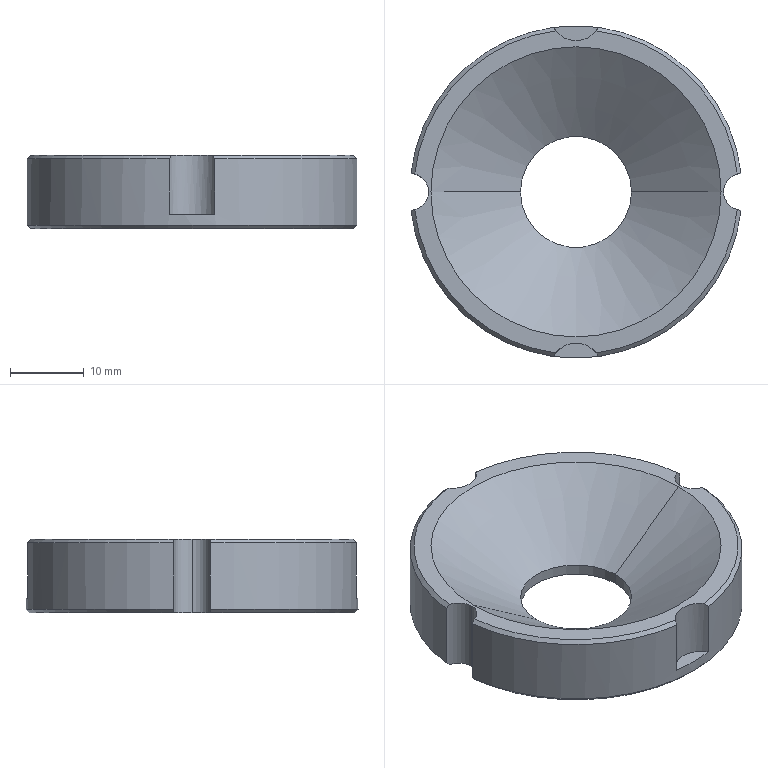Part | STEP file | 10000020561swp000-1 | 1 solid | 21 faces | box 44.722 x 45 x 10 mm | volume 10014 mm3 | cylinder 9 | cone 8 | plane 4 | commonest cylinder face diameters 5 x3 7 x2 15.05 x2 45 x2
STEP:
#1=CARTESIAN_POINT('',(7.525,0.,1.5));
#2=VERTEX_POINT('',#1);
#3=CARTESIAN_POINT('',(-7.525,0.,1.5));
#4=VERTEX_POINT('',#3);
#5=CARTESIAN_POINT('',(0.,0.,1.5));
#6=DIRECTION('',(0.,0.,-1.));
#7=DIRECTION('',(-1.,0.,0.));
#8=AXIS2_PLACEMENT_3D('',#5,#6,#7);
#9=CIRCLE('',#8,7.525);
#10=EDGE_CURVE('',#2,#4,#9,.T.);
#11=ORIENTED_EDGE('',*,*,#10,.T.);
#12=CARTESIAN_POINT('',(-19.664,0.,10.));
#13=VERTEX_POINT('',#12);
#14=CARTESIAN_POINT('',(-7.525,0.,1.5));
#15=DIRECTION('',(-0.8192,0.,0.5736));
#16=VECTOR('',#15,1000.);
#17=LINE('',#14,#16);
#18=EDGE_CURVE('',#4,#13,#17,.T.);
#19=ORIENTED_EDGE('',*,*,#18,.T.);
#20=CARTESIAN_POINT('',(19.664,0.,10.));
#21=VERTEX_POINT('',#20);
#22=CARTESIAN_POINT('',(0.,0.,10.));
#23=DIRECTION('',(0.,0.,-1.));
#24=DIRECTION('',(-1.,0.,0.));
#25=AXIS2_PLACEMENT_3D('',#22,#23,#24);
#26=CIRCLE('',#25,19.664);
#27=EDGE_CURVE('',#21,#13,#26,.T.);
#28=ORIENTED_EDGE('',*,*,#27,.F.);
#29=CARTESIAN_POINT('',(7.525,0.,1.5));
#30=DIRECTION('',(0.8192,0.,0.5736));
#31=VECTOR('',#30,1000.);
#32=LINE('',#29,#31);
#33=EDGE_CURVE('',#2,#21,#32,.T.);
#34=ORIENTED_EDGE('',*,*,#33,.F.);
#35=EDGE_LOOP('',(#11,#19,#28,#34));
#36=FACE_OUTER_BOUND('',#35,.T.);
#37=CARTESIAN_POINT('',(0.,0.,1.5));
#38=DIRECTION('',(0.,0.,1.));
#39=DIRECTION('',(1.,0.,0.));
#40=AXIS2_PLACEMENT_3D('',#37,#38,#39);
#41=CONICAL_SURFACE('',#40,7.525,0.9599);
#42=ADVANCED_FACE('',(#36),#41,.F.);
#43=CARTESIAN_POINT('',(-20.,0.,0.));
#44=VERTEX_POINT('',#43);
#45=CARTESIAN_POINT('',(-21.867,2.418,0.));
#46=VERTEX_POINT('',#45);
#47=CARTESIAN_POINT('',(-22.5,0.,0.));
#48=DIRECTION('',(0.,0.,1.));
#49=DIRECTION('',(1.,0.,0.));
#50=AXIS2_PLACEMENT_3D('',#47,#48,#49);
#51=CIRCLE('',#50,2.5);
#52=EDGE_CURVE('',#44,#46,#51,.T.);
#53=ORIENTED_EDGE('',*,*,#52,.F.);
#54=CARTESIAN_POINT('',(-20.,0.,10.));
#55=VERTEX_POINT('',#54);
#56=CARTESIAN_POINT('',(-20.,0.,0.));
#57=DIRECTION('',(0.,0.,1.));
#58=VECTOR('',#57,1000.);
#59=LINE('',#56,#58);
#60=EDGE_CURVE('',#44,#55,#59,.T.);
#61=ORIENTED_EDGE('',*,*,#60,.T.);
#62=CARTESIAN_POINT('',(-21.867,2.418,10.));
#63=VERTEX_POINT('',#62);
#64=CARTESIAN_POINT('',(-22.5,0.,10.));
#65=DIRECTION('',(0.,0.,1.));
#66=DIRECTION('',(1.,0.,0.));
#67=AXIS2_PLACEMENT_3D('',#64,#65,#66);
#68=CIRCLE('',#67,2.5);
#69=EDGE_CURVE('',#55,#63,#68,.T.);
#70=ORIENTED_EDGE('',*,*,#69,.T.);
#71=CARTESIAN_POINT('',(-22.361,2.496,9.5));
#72=VERTEX_POINT('',#71);
#73=CARTESIAN_POINT('',(-21.867,2.418,10.));
#74=CARTESIAN_POINT('',(-22.029,2.461,9.834));
#75=CARTESIAN_POINT('',(-22.194,2.487,9.667));
#76=CARTESIAN_POINT('',(-22.361,2.496,9.5));
#77=B_SPLINE_CURVE_WITH_KNOTS('',3,(#73,#74,#75,#76),.UNSPECIFIED.,.F.,.F.,(4,4),(0.,0.0007075),.UNSPECIFIED.);
#78=EDGE_CURVE('',#63,#72,#77,.T.);
#79=ORIENTED_EDGE('',*,*,#78,.T.);
#80=CARTESIAN_POINT('',(-22.361,2.496,0.5));
#81=VERTEX_POINT('',#80);
#82=CARTESIAN_POINT('',(-22.361,2.496,5.));
#83=DIRECTION('',(0.,0.,1.));
#84=VECTOR('',#83,1000.);
#85=LINE('',#82,#84);
#86=EDGE_CURVE('',#81,#72,#85,.T.);
#87=ORIENTED_EDGE('',*,*,#86,.F.);
#88=CARTESIAN_POINT('',(-22.361,2.496,0.5));
#89=CARTESIAN_POINT('',(-22.194,2.487,0.333));
#90=CARTESIAN_POINT('',(-22.029,2.461,0.1663));
#91=CARTESIAN_POINT('',(-21.867,2.418,0.));
#92=B_SPLINE_CURVE_WITH_KNOTS('',3,(#88,#89,#90,#91),.UNSPECIFIED.,.F.,.F.,(4,4),(0.,0.0007075),.UNSPECIFIED.);
#93=EDGE_CURVE('',#81,#46,#92,.T.);
#94=ORIENTED_EDGE('',*,*,#93,.T.);
#95=EDGE_LOOP('',(#53,#61,#70,#79,#87,#94));
#96=FACE_OUTER_BOUND('',#95,.T.);
#97=CARTESIAN_POINT('',(-22.5,0.,0.));
#98=DIRECTION('',(0.,0.,1.));
#99=DIRECTION('',(1.,0.,0.));
#100=AXIS2_PLACEMENT_3D('',#97,#98,#99);
#101=CYLINDRICAL_SURFACE('',#100,2.5);
#102=ADVANCED_FACE('',(#96),#101,.F.);
#103=ORIENTED_EDGE('',*,*,#10,.F.);
#104=CARTESIAN_POINT('',(7.525,0.,0.));
#105=VERTEX_POINT('',#104);
#106=CARTESIAN_POINT('',(7.525,0.,10.));
#107=DIRECTION('',(0.,0.,-1.));
#108=VECTOR('',#107,1000.);
#109=LINE('',#106,#108);
#110=EDGE_CURVE('',#2,#105,#109,.T.);
#111=ORIENTED_EDGE('',*,*,#110,.T.);
#112=CARTESIAN_POINT('',(-7.525,0.,0.));
#113=VERTEX_POINT('',#112);
#114=CARTESIAN_POINT('',(0.,0.,0.));
#115=DIRECTION('',(0.,0.,1.));
#116=DIRECTION('',(1.,0.,0.));
#117=AXIS2_PLACEMENT_3D('',#114,#115,#116);
#118=CIRCLE('',#117,7.525);
#119=EDGE_CURVE('',#113,#105,#118,.T.);
#120=ORIENTED_EDGE('',*,*,#119,.F.);
#121=CARTESIAN_POINT('',(-7.525,0.,10.));
#122=DIRECTION('',(0.,0.,-1.));
#123=VECTOR('',#122,1000.);
#124=LINE('',#121,#123);
#125=EDGE_CURVE('',#4,#113,#124,.T.);
#126=ORIENTED_EDGE('',*,*,#125,.F.);
#127=EDGE_LOOP('',(#103,#111,#120,#126));
#128=FACE_OUTER_BOUND('',#127,.T.);
#129=CARTESIAN_POINT('',(0.,0.,10.));
#130=DIRECTION('',(0.,0.,-1.));
#131=DIRECTION('',(-1.,0.,0.));
#132=AXIS2_PLACEMENT_3D('',#129,#130,#131);
#133=CYLINDRICAL_SURFACE('',#132,7.525);
#134=ADVANCED_FACE('',(#128),#133,.F.);
#135=CARTESIAN_POINT('',(22.361,2.496,9.5));
#136=VERTEX_POINT('',#135);
#137=CARTESIAN_POINT('',(22.361,2.496,0.5));
#138=VERTEX_POINT('',#137);
#139=CARTESIAN_POINT('',(22.361,2.496,5.));
#140=DIRECTION('',(0.,0.,-1.));
#141=VECTOR('',#140,1000.);
#142=LINE('',#139,#141);
#143=EDGE_CURVE('',#136,#138,#142,.T.);
#144=ORIENTED_EDGE('',*,*,#143,.T.);
#145=CARTESIAN_POINT('',(0.,0.,0.5));
#146=DIRECTION('',(0.,0.,1.));
#147=DIRECTION('',(1.,0.,0.));
#148=AXIS2_PLACEMENT_3D('',#145,#146,#147);
#149=CIRCLE('',#148,22.5);
#150=EDGE_CURVE('',#138,#81,#149,.T.);
#151=ORIENTED_EDGE('',*,*,#150,.T.);
#152=ORIENTED_EDGE('',*,*,#86,.T.);
#153=CARTESIAN_POINT('',(-3.055,22.292,9.5));
#154=VERTEX_POINT('',#153);
#155=CARTESIAN_POINT('',(0.,0.,9.5));
#156=DIRECTION('',(0.,0.,-1.));
#157=DIRECTION('',(1.,0.,0.));
#158=AXIS2_PLACEMENT_3D('',#155,#156,#157);
#159=CIRCLE('',#158,22.5);
#160=EDGE_CURVE('',#72,#154,#159,.T.);
#161=ORIENTED_EDGE('',*,*,#160,.T.);
#162=CARTESIAN_POINT('',(-3.055,22.292,2.));
#163=VERTEX_POINT('',#162);
#164=CARTESIAN_POINT('',(-3.055,22.292,6.));
#165=DIRECTION('',(0.,0.,-1.));
#166=VECTOR('',#165,1000.);
#167=LINE('',#164,#166);
#168=EDGE_CURVE('',#154,#163,#167,.T.);
#169=ORIENTED_EDGE('',*,*,#168,.T.);
#170=CARTESIAN_POINT('',(3.055,22.292,2.));
#171=VERTEX_POINT('',#170);
#172=CARTESIAN_POINT('',(0.,0.,2.));
#173=DIRECTION('',(0.,0.,1.));
#174=DIRECTION('',(1.,0.,0.));
#175=AXIS2_PLACEMENT_3D('',#172,#173,#174);
#176=CIRCLE('',#175,22.5);
#177=EDGE_CURVE('',#171,#163,#176,.T.);
#178=ORIENTED_EDGE('',*,*,#177,.F.);
#179=CARTESIAN_POINT('',(3.055,22.292,9.5));
#180=VERTEX_POINT('',#179);
#181=CARTESIAN_POINT('',(3.055,22.292,6.));
#182=DIRECTION('',(0.,0.,1.));
#183=VECTOR('',#182,1000.);
#184=LINE('',#181,#183);
#185=EDGE_CURVE('',#171,#180,#184,.T.);
#186=ORIENTED_EDGE('',*,*,#185,.T.);
#187=CARTESIAN_POINT('',(0.,0.,9.5));
#188=DIRECTION('',(0.,0.,-1.));
#189=DIRECTION('',(1.,0.,0.));
#190=AXIS2_PLACEMENT_3D('',#187,#188,#189);
#191=CIRCLE('',#190,22.5);
#192=EDGE_CURVE('',#180,#136,#191,.T.);
#193=ORIENTED_EDGE('',*,*,#192,.T.);
#194=EDGE_LOOP('',(#144,#151,#152,#161,#169,#178,#186,#193));
#195=FACE_OUTER_BOUND('',#194,.T.);
#196=CARTESIAN_POINT('',(0.,0.,10.));
#197=DIRECTION('',(0.,0.,-1.));
#198=DIRECTION('',(-1.,0.,0.));
#199=AXIS2_PLACEMENT_3D('',#196,#197,#198);
#200=CYLINDRICAL_SURFACE('',#199,22.5);
#201=ADVANCED_FACE('',(#195),#200,.T.);
#202=ORIENTED_EDGE('',*,*,#27,.T.);
#203=CARTESIAN_POINT('',(0.,0.,10.));
#204=DIRECTION('',(0.,0.,-1.));
#205=DIRECTION('',(-1.,0.,0.));
#206=AXIS2_PLACEMENT_3D('',#203,#204,#205);
#207=CIRCLE('',#206,19.664);
#208=EDGE_CURVE('',#13,#21,#207,.T.);
#209=ORIENTED_EDGE('',*,*,#208,.T.);
#210=EDGE_LOOP('',(#202,#209));
#211=FACE_BOUND('',#210,.T.);
#212=CARTESIAN_POINT('',(2.745,-21.828,10.));
#213=VERTEX_POINT('',#212);
#214=CARTESIAN_POINT('',(-2.745,-21.828,10.));
#215=VERTEX_POINT('',#214);
#216=CARTESIAN_POINT('',(0.,-24.,10.));
#217=DIRECTION('',(0.,0.,1.));
#218=DIRECTION('',(1.,0.,0.));
#219=AXIS2_PLACEMENT_3D('',#216,#217,#218);
#220=CIRCLE('',#219,3.5);
#221=EDGE_CURVE('',#213,#215,#220,.T.);
#222=ORIENTED_EDGE('',*,*,#221,.F.);
#223=CARTESIAN_POINT('',(21.867,-2.418,10.));
#224=VERTEX_POINT('',#223);
#225=CARTESIAN_POINT('',(0.,0.,10.));
#226=DIRECTION('',(0.,0.,1.));
#227=DIRECTION('',(1.,0.,0.));
#228=AXIS2_PLACEMENT_3D('',#225,#226,#227);
#229=CIRCLE('',#228,22.);
#230=EDGE_CURVE('',#213,#224,#229,.T.);
#231=ORIENTED_EDGE('',*,*,#230,.T.);
#232=CARTESIAN_POINT('',(21.867,2.418,10.));
#233=VERTEX_POINT('',#232);
#234=CARTESIAN_POINT('',(22.5,0.,10.));
#235=DIRECTION('',(0.,0.,1.));
#236=DIRECTION('',(1.,0.,0.));
#237=AXIS2_PLACEMENT_3D('',#234,#235,#236);
#238=CIRCLE('',#237,2.5);
#239=EDGE_CURVE('',#233,#224,#238,.T.);
#240=ORIENTED_EDGE('',*,*,#239,.F.);
#241=CARTESIAN_POINT('',(2.745,21.828,10.));
#242=VERTEX_POINT('',#241);
#243=CARTESIAN_POINT('',(0.,0.,10.));
#244=DIRECTION('',(0.,0.,1.));
#245=DIRECTION('',(1.,0.,0.));
#246=AXIS2_PLACEMENT_3D('',#243,#244,#245);
#247=CIRCLE('',#246,22.);
#248=EDGE_CURVE('',#233,#242,#247,.T.);
#249=ORIENTED_EDGE('',*,*,#248,.T.);
#250=CARTESIAN_POINT('',(-2.745,21.828,10.));
#251=VERTEX_POINT('',#250);
#252=CARTESIAN_POINT('',(0.,24.,10.));
#253=DIRECTION('',(0.,0.,1.));
#254=DIRECTION('',(1.,0.,0.));
#255=AXIS2_PLACEMENT_3D('',#252,#253,#254);
#256=CIRCLE('',#255,3.5);
#257=EDGE_CURVE('',#251,#242,#256,.T.);
#258=ORIENTED_EDGE('',*,*,#257,.F.);
#259=CARTESIAN_POINT('',(0.,0.,10.));
#260=DIRECTION('',(0.,0.,1.));
#261=DIRECTION('',(1.,0.,0.));
#262=AXIS2_PLACEMENT_3D('',#259,#260,#261);
#263=CIRCLE('',#262,22.);
#264=EDGE_CURVE('',#251,#63,#263,.T.);
#265=ORIENTED_EDGE('',*,*,#264,.T.);
#266=ORIENTED_EDGE('',*,*,#69,.F.);
#267=CARTESIAN_POINT('',(-21.867,-2.418,10.));
#268=VERTEX_POINT('',#267);
#269=CARTESIAN_POINT('',(-22.5,0.,10.));
#270=DIRECTION('',(0.,0.,1.));
#271=DIRECTION('',(1.,0.,0.));
#272=AXIS2_PLACEMENT_3D('',#269,#270,#271);
#273=CIRCLE('',#272,2.5);
#274=EDGE_CURVE('',#268,#55,#273,.T.);
#275=ORIENTED_EDGE('',*,*,#274,.F.);
#276=CARTESIAN_POINT('',(0.,0.,10.));
#277=DIRECTION('',(0.,0.,1.));
#278=DIRECTION('',(1.,0.,0.));
#279=AXIS2_PLACEMENT_3D('',#276,#277,#278);
#280=CIRCLE('',#279,22.);
#281=EDGE_CURVE('',#268,#215,#280,.T.);
#282=ORIENTED_EDGE('',*,*,#281,.T.);
#283=EDGE_LOOP('',(#222,#231,#240,#249,#258,#265,#266,#275,#282));
#284=FACE_OUTER_BOUND('',#283,.T.);
#285=CARTESIAN_POINT('',(0.,0.,10.));
#286=DIRECTION('',(0.,0.,1.));
#287=DIRECTION('',(1.,0.,0.));
#288=AXIS2_PLACEMENT_3D('',#285,#286,#287);
#289=PLANE('',#288);
#290=ADVANCED_FACE('',(#211,#284),#289,.T.);
#291=CARTESIAN_POINT('',(21.867,2.418,0.));
#292=VERTEX_POINT('',#291);
#293=CARTESIAN_POINT('',(21.867,-2.418,0.));
#294=VERTEX_POINT('',#293);
#295=CARTESIAN_POINT('',(22.5,0.,0.));
#296=DIRECTION('',(0.,0.,1.));
#297=DIRECTION('',(1.,0.,0.));
#298=AXIS2_PLACEMENT_3D('',#295,#296,#297);
#299=CIRCLE('',#298,2.5);
#300=EDGE_CURVE('',#292,#294,#299,.T.);
#301=ORIENTED_EDGE('',*,*,#300,.T.);
#302=CARTESIAN_POINT('',(-21.867,-2.418,0.));
#303=VERTEX_POINT('',#302);
#304=CARTESIAN_POINT('',(0.,0.,0.));
#305=DIRECTION('',(0.,0.,-1.));
#306=DIRECTION('',(1.,0.,0.));
#307=AXIS2_PLACEMENT_3D('',#304,#305,#306);
#308=CIRCLE('',#307,22.);
#309=EDGE_CURVE('',#294,#303,#308,.T.);
#310=ORIENTED_EDGE('',*,*,#309,.T.);
#311=CARTESIAN_POINT('',(-22.5,0.,0.));
#312=DIRECTION('',(0.,0.,1.));
#313=DIRECTION('',(1.,0.,0.));
#314=AXIS2_PLACEMENT_3D('',#311,#312,#313);
#315=CIRCLE('',#314,2.5);
#316=EDGE_CURVE('',#303,#44,#315,.T.);
#317=ORIENTED_EDGE('',*,*,#316,.T.);
#318=ORIENTED_EDGE('',*,*,#52,.T.);
#319=CARTESIAN_POINT('',(0.,0.,0.));
#320=DIRECTION('',(0.,0.,-1.));
#321=DIRECTION('',(1.,0.,0.));
#322=AXIS2_PLACEMENT_3D('',#319,#320,#321);
#323=CIRCLE('',#322,22.);
#324=EDGE_CURVE('',#46,#292,#323,.T.);
#325=ORIENTED_EDGE('',*,*,#324,.T.);
#326=EDGE_LOOP('',(#301,#310,#317,#318,#325));
#327=FACE_OUTER_BOUND('',#326,.T.);
#328=ORIENTED_EDGE('',*,*,#119,.T.);
#329=CARTESIAN_POINT('',(0.,0.,0.));
#330=DIRECTION('',(0.,0.,1.));
#331=DIRECTION('',(1.,0.,0.));
#332=AXIS2_PLACEMENT_3D('',#329,#330,#331);
#333=CIRCLE('',#332,7.525);
#334=EDGE_CURVE('',#105,#113,#333,.T.);
#335=ORIENTED_EDGE('',*,*,#334,.T.);
#336=EDGE_LOOP('',(#328,#335));
#337=FACE_BOUND('',#336,.T.);
#338=CARTESIAN_POINT('',(0.,0.,0.));
#339=DIRECTION('',(0.,0.,1.));
#340=DIRECTION('',(1.,0.,0.));
#341=AXIS2_PLACEMENT_3D('',#338,#339,#340);
#342=PLANE('',#341);
#343=ADVANCED_FACE('',(#327,#337),#342,.F.);
#344=CARTESIAN_POINT('',(-22.361,-2.496,9.5));
#345=VERTEX_POINT('',#344);
#346=CARTESIAN_POINT('',(-22.361,-2.496,0.5));
#347=VERTEX_POINT('',#346);
#348=CARTESIAN_POINT('',(-22.361,-2.496,5.));
#349=DIRECTION('',(0.,0.,-1.));
#350=VECTOR('',#349,1000.);
#351=LINE('',#348,#350);
#352=EDGE_CURVE('',#345,#347,#351,.T.);
#353=ORIENTED_EDGE('',*,*,#352,.T.);
#354=CARTESIAN_POINT('',(22.361,-2.496,0.5));
#355=VERTEX_POINT('',#354);
#356=CARTESIAN_POINT('',(0.,0.,0.5));
#357=DIRECTION('',(0.,0.,1.));
#358=DIRECTION('',(1.,0.,0.));
#359=AXIS2_PLACEMENT_3D('',#356,#357,#358);
#360=CIRCLE('',#359,22.5);
#361=EDGE_CURVE('',#347,#355,#360,.T.);
#362=ORIENTED_EDGE('',*,*,#361,.T.);
#363=CARTESIAN_POINT('',(22.361,-2.496,9.5));
#364=VERTEX_POINT('',#363);
#365=CARTESIAN_POINT('',(22.361,-2.496,5.));
#366=DIRECTION('',(0.,0.,1.));
#367=VECTOR('',#366,1000.);
#368=LINE('',#365,#367);
#369=EDGE_CURVE('',#355,#364,#368,.T.);
#370=ORIENTED_EDGE('',*,*,#369,.T.);
#371=CARTESIAN_POINT('',(3.055,-22.292,9.5));
#372=VERTEX_POINT('',#371);
#373=CARTESIAN_POINT('',(0.,0.,9.5));
#374=DIRECTION('',(0.,0.,-1.));
#375=DIRECTION('',(1.,0.,0.));
#376=AXIS2_PLACEMENT_3D('',#373,#374,#375);
#377=CIRCLE('',#376,22.5);
#378=EDGE_CURVE('',#364,#372,#377,.T.);
#379=ORIENTED_EDGE('',*,*,#378,.T.);
#380=CARTESIAN_POINT('',(3.055,-22.292,2.));
#381=VERTEX_POINT('',#380);
#382=CARTESIAN_POINT('',(3.055,-22.292,6.));
#383=DIRECTION('',(0.,0.,-1.));
#384=VECTOR('',#383,1000.);
#385=LINE('',#382,#384);
#386=EDGE_CURVE('',#372,#381,#385,.T.);
#387=ORIENTED_EDGE('',*,*,#386,.T.);
#388=CARTESIAN_POINT('',(-3.055,-22.292,2.));
#389=VERTEX_POINT('',#388);
#390=CARTESIAN_POINT('',(0.,0.,2.));
#391=DIRECTION('',(0.,0.,1.));
#392=DIRECTION('',(1.,0.,0.));
#393=AXIS2_PLACEMENT_3D('',#390,#391,#392);
#394=CIRCLE('',#393,22.5);
#395=EDGE_CURVE('',#389,#381,#394,.T.);
#396=ORIENTED_EDGE('',*,*,#395,.F.);
#397=CARTESIAN_POINT('',(-3.055,-22.292,9.5));
#398=VERTEX_POINT('',#397);
#399=CARTESIAN_POINT('',(-3.055,-22.292,6.));
#400=DIRECTION('',(0.,0.,1.));
#401=VECTOR('',#400,1000.);
#402=LINE('',#399,#401);
#403=EDGE_CURVE('',#389,#398,#402,.T.);
#404=ORIENTED_EDGE('',*,*,#403,.T.);
#405=CARTESIAN_POINT('',(0.,0.,9.5));
#406=DIRECTION('',(0.,0.,-1.));
#407=DIRECTION('',(1.,0.,0.));
#408=AXIS2_PLACEMENT_3D('',#405,#406,#407);
#409=CIRCLE('',#408,22.5);
#410=EDGE_CURVE('',#398,#345,#409,.T.);
#411=ORIENTED_EDGE('',*,*,#410,.T.);
#412=EDGE_LOOP('',(#353,#362,#370,#379,#387,#396,#404,#411));
#413=FACE_OUTER_BOUND('',#412,.T.);
#414=CARTESIAN_POINT('',(0.,0.,10.));
#415=DIRECTION('',(0.,0.,-1.));
#416=DIRECTION('',(-1.,0.,0.));
#417=AXIS2_PLACEMENT_3D('',#414,#415,#416);
#418=CYLINDRICAL_SURFACE('',#417,22.5);
#419=ADVANCED_FACE('',(#413),#418,.T.);
#420=ORIENTED_EDGE('',*,*,#110,.F.);
#421=CARTESIAN_POINT('',(0.,0.,1.5));
#422=DIRECTION('',(0.,0.,-1.));
#423=DIRECTION('',(-1.,0.,0.));
#424=AXIS2_PLACEMENT_3D('',#421,#422,#423);
#425=CIRCLE('',#424,7.525);
#426=EDGE_CURVE('',#4,#2,#425,.T.);
#427=ORIENTED_EDGE('',*,*,#426,.F.);
#428=ORIENTED_EDGE('',*,*,#125,.T.);
#429=ORIENTED_EDGE('',*,*,#334,.F.);
#430=EDGE_LOOP('',(#420,#427,#428,#429));
#431=FACE_OUTER_BOUND('',#430,.T.);
#432=CARTESIAN_POINT('',(0.,0.,10.));
#433=DIRECTION('',(0.,0.,-1.));
#434=DIRECTION('',(-1.,0.,0.));
#435=AXIS2_PLACEMENT_3D('',#432,#433,#434);
#436=CYLINDRICAL_SURFACE('',#435,7.525);
#437=ADVANCED_FACE('',(#431),#436,.F.);
#438=ORIENTED_EDGE('',*,*,#369,.F.);
#439=CARTESIAN_POINT('',(22.361,-2.496,0.5));
#440=CARTESIAN_POINT('',(22.194,-2.487,0.333));
#441=CARTESIAN_POINT('',(22.029,-2.461,0.1663));
#442=CARTESIAN_POINT('',(21.867,-2.418,0.));
#443=B_SPLINE_CURVE_WITH_KNOTS('',3,(#439,#440,#441,#442),.UNSPECIFIED.,.F.,.F.,(4,4),(0.,0.0007075),.UNSPECIFIED.);
#444=EDGE_CURVE('',#355,#294,#443,.T.);
#445=ORIENTED_EDGE('',*,*,#444,.T.);
#446=ORIENTED_EDGE('',*,*,#300,.F.);
#447=CARTESIAN_POINT('',(21.867,2.418,0.));
#448=CARTESIAN_POINT('',(22.029,2.461,0.1663));
#449=CARTESIAN_POINT('',(22.194,2.487,0.333));
#450=CARTESIAN_POINT('',(22.361,2.496,0.5));
#451=B_SPLINE_CURVE_WITH_KNOTS('',3,(#447,#448,#449,#450),.UNSPECIFIED.,.F.,.F.,(4,4),(0.,0.0007075),.UNSPECIFIED.);
#452=EDGE_CURVE('',#292,#138,#451,.T.);
#453=ORIENTED_EDGE('',*,*,#452,.T.);
#454=ORIENTED_EDGE('',*,*,#143,.F.);
#455=CARTESIAN_POINT('',(22.361,2.496,9.5));
#456=CARTESIAN_POINT('',(22.194,2.487,9.667));
#457=CARTESIAN_POINT('',(22.029,2.461,9.834));
#458=CARTESIAN_POINT('',(21.867,2.418,10.));
#459=B_SPLINE_CURVE_WITH_KNOTS('',3,(#455,#456,#457,#458),.UNSPECIFIED.,.F.,.F.,(4,4),(0.,0.0007075),.UNSPECIFIED.);
#460=EDGE_CURVE('',#136,#233,#459,.T.);
#461=ORIENTED_EDGE('',*,*,#460,.T.);
#462=ORIENTED_EDGE('',*,*,#239,.T.);
#463=CARTESIAN_POINT('',(21.867,-2.418,10.));
#464=CARTESIAN_POINT('',(22.029,-2.461,9.834));
#465=CARTESIAN_POINT('',(22.194,-2.487,9.667));
#466=CARTESIAN_POINT('',(22.361,-2.496,9.5));
#467=B_SPLINE_CURVE_WITH_KNOTS('',3,(#463,#464,#465,#466),.UNSPECIFIED.,.F.,.F.,(4,4),(0.,0.0007075),.UNSPECIFIED.);
#468=EDGE_CURVE('',#224,#364,#467,.T.);
#469=ORIENTED_EDGE('',*,*,#468,.T.);
#470=EDGE_LOOP('',(#438,#445,#446,#453,#454,#461,#462,#469));
#471=FACE_OUTER_BOUND('',#470,.T.);
#472=CARTESIAN_POINT('',(22.5,0.,0.));
#473=DIRECTION('',(0.,0.,1.));
#474=DIRECTION('',(1.,0.,0.));
#475=AXIS2_PLACEMENT_3D('',#472,#473,#474);
#476=CYLINDRICAL_SURFACE('',#475,2.5);
#477=ADVANCED_FACE('',(#471),#476,.F.);
#478=ORIENTED_EDGE('',*,*,#60,.F.);
#479=ORIENTED_EDGE('',*,*,#316,.F.);
#480=CARTESIAN_POINT('',(-21.867,-2.418,0.));
#481=CARTESIAN_POINT('',(-22.029,-2.461,0.1663));
#482=CARTESIAN_POINT('',(-22.194,-2.487,0.333));
#483=CARTESIAN_POINT('',(-22.361,-2.496,0.5));
#484=B_SPLINE_CURVE_WITH_KNOTS('',3,(#480,#481,#482,#483),.UNSPECIFIED.,.F.,.F.,(4,4),(0.,0.0007075),.UNSPECIFIED.);
#485=EDGE_CURVE('',#303,#347,#484,.T.);
#486=ORIENTED_EDGE('',*,*,#485,.T.);
#487=ORIENTED_EDGE('',*,*,#352,.F.);
#488=CARTESIAN_POINT('',(-22.361,-2.496,9.5));
#489=CARTESIAN_POINT('',(-22.194,-2.487,9.667));
#490=CARTESIAN_POINT('',(-22.029,-2.461,9.834));
#491=CARTESIAN_POINT('',(-21.867,-2.418,10.));
#492=B_SPLINE_CURVE_WITH_KNOTS('',3,(#488,#489,#490,#491),.UNSPECIFIED.,.F.,.F.,(4,4),(0.,0.0007075),.UNSPECIFIED.);
#493=EDGE_CURVE('',#345,#268,#492,.T.);
#494=ORIENTED_EDGE('',*,*,#493,.T.);
#495=ORIENTED_EDGE('',*,*,#274,.T.);
#496=EDGE_LOOP('',(#478,#479,#486,#487,#494,#495));
#497=FACE_OUTER_BOUND('',#496,.T.);
#498=CARTESIAN_POINT('',(-22.5,0.,0.));
#499=DIRECTION('',(0.,0.,1.));
#500=DIRECTION('',(1.,0.,0.));
#501=AXIS2_PLACEMENT_3D('',#498,#499,#500);
#502=CYLINDRICAL_SURFACE('',#501,2.5);
#503=ADVANCED_FACE('',(#497),#502,.F.);
#504=ORIENTED_EDGE('',*,*,#177,.T.);
#505=CARTESIAN_POINT('',(0.,24.,2.));
#506=DIRECTION('',(0.,0.,1.));
#507=DIRECTION('',(1.,0.,0.));
#508=AXIS2_PLACEMENT_3D('',#505,#506,#507);
#509=CIRCLE('',#508,3.5);
#510=EDGE_CURVE('',#163,#171,#509,.T.);
#511=ORIENTED_EDGE('',*,*,#510,.T.);
#512=EDGE_LOOP('',(#504,#511));
#513=FACE_OUTER_BOUND('',#512,.T.);
#514=CARTESIAN_POINT('',(0.,24.,2.));
#515=DIRECTION('',(0.,0.,1.));
#516=DIRECTION('',(1.,0.,0.));
#517=AXIS2_PLACEMENT_3D('',#514,#515,#516);
#518=PLANE('',#517);
#519=ADVANCED_FACE('',(#513),#518,.T.);
#520=ORIENTED_EDGE('',*,*,#257,.T.);
#521=CARTESIAN_POINT('',(2.745,21.828,10.));
#522=CARTESIAN_POINT('',(2.863,21.977,9.837));
#523=CARTESIAN_POINT('',(2.965,22.132,9.67));
#524=CARTESIAN_POINT('',(3.055,22.292,9.5));
#525=B_SPLINE_CURVE_WITH_KNOTS('',3,(#521,#522,#523,#524),.UNSPECIFIED.,.F.,.F.,(4,4),(0.,0.000749),.UNSPECIFIED.);
#526=EDGE_CURVE('',#242,#180,#525,.T.);
#527=ORIENTED_EDGE('',*,*,#526,.T.);
#528=ORIENTED_EDGE('',*,*,#185,.F.);
#529=ORIENTED_EDGE('',*,*,#510,.F.);
#530=ORIENTED_EDGE('',*,*,#168,.F.);
#531=CARTESIAN_POINT('',(-3.055,22.292,9.5));
#532=CARTESIAN_POINT('',(-2.965,22.132,9.67));
#533=CARTESIAN_POINT('',(-2.863,21.977,9.837));
#534=CARTESIAN_POINT('',(-2.745,21.828,10.));
#535=B_SPLINE_CURVE_WITH_KNOTS('',3,(#531,#532,#533,#534),.UNSPECIFIED.,.F.,.F.,(4,4),(0.,0.000749),.UNSPECIFIED.);
#536=EDGE_CURVE('',#154,#251,#535,.T.);
#537=ORIENTED_EDGE('',*,*,#536,.T.);
#538=EDGE_LOOP('',(#520,#527,#528,#529,#530,#537));
#539=FACE_OUTER_BOUND('',#538,.T.);
#540=CARTESIAN_POINT('',(0.,24.,2.));
#541=DIRECTION('',(0.,0.,1.));
#542=DIRECTION('',(1.,0.,0.));
#543=AXIS2_PLACEMENT_3D('',#540,#541,#542);
#544=CYLINDRICAL_SURFACE('',#543,3.5);
#545=ADVANCED_FACE('',(#539),#544,.F.);
#546=ORIENTED_EDGE('',*,*,#386,.F.);
#547=CARTESIAN_POINT('',(3.055,-22.292,9.5));
#548=CARTESIAN_POINT('',(2.965,-22.132,9.67));
#549=CARTESIAN_POINT('',(2.863,-21.977,9.837));
#550=CARTESIAN_POINT('',(2.745,-21.828,10.));
#551=B_SPLINE_CURVE_WITH_KNOTS('',3,(#547,#548,#549,#550),.UNSPECIFIED.,.F.,.F.,(4,4),(0.,0.000749),.UNSPECIFIED.);
#552=EDGE_CURVE('',#372,#213,#551,.T.);
#553=ORIENTED_EDGE('',*,*,#552,.T.);
#554=ORIENTED_EDGE('',*,*,#221,.T.);
#555=CARTESIAN_POINT('',(-2.745,-21.828,10.));
#556=CARTESIAN_POINT('',(-2.863,-21.977,9.837));
#557=CARTESIAN_POINT('',(-2.965,-22.132,9.67));
#558=CARTESIAN_POINT('',(-3.055,-22.292,9.5));
#559=B_SPLINE_CURVE_WITH_KNOTS('',3,(#555,#556,#557,#558),.UNSPECIFIED.,.F.,.F.,(4,4),(0.,0.000749),.UNSPECIFIED.);
#560=EDGE_CURVE('',#215,#398,#559,.T.);
#561=ORIENTED_EDGE('',*,*,#560,.T.);
#562=ORIENTED_EDGE('',*,*,#403,.F.);
#563=CARTESIAN_POINT('',(0.,-24.,2.));
#564=DIRECTION('',(0.,0.,1.));
#565=DIRECTION('',(1.,0.,0.));
#566=AXIS2_PLACEMENT_3D('',#563,#564,#565);
#567=CIRCLE('',#566,3.5);
#568=EDGE_CURVE('',#381,#389,#567,.T.);
#569=ORIENTED_EDGE('',*,*,#568,.F.);
#570=EDGE_LOOP('',(#546,#553,#554,#561,#562,#569));
#571=FACE_OUTER_BOUND('',#570,.T.);
#572=CARTESIAN_POINT('',(0.,-24.,2.));
#573=DIRECTION('',(0.,0.,1.));
#574=DIRECTION('',(1.,0.,0.));
#575=AXIS2_PLACEMENT_3D('',#572,#573,#574);
#576=CYLINDRICAL_SURFACE('',#575,3.5);
#577=ADVANCED_FACE('',(#571),#576,.F.);
#578=ORIENTED_EDGE('',*,*,#395,.T.);
#579=ORIENTED_EDGE('',*,*,#568,.T.);
#580=EDGE_LOOP('',(#578,#579));
#581=FACE_OUTER_BOUND('',#580,.T.);
#582=CARTESIAN_POINT('',(0.,-24.,2.));
#583=DIRECTION('',(0.,0.,1.));
#584=DIRECTION('',(1.,0.,0.));
#585=AXIS2_PLACEMENT_3D('',#582,#583,#584);
#586=PLANE('',#585);
#587=ADVANCED_FACE('',(#581),#586,.T.);
#588=ORIENTED_EDGE('',*,*,#18,.F.);
#589=ORIENTED_EDGE('',*,*,#426,.T.);
#590=ORIENTED_EDGE('',*,*,#33,.T.);
#591=ORIENTED_EDGE('',*,*,#208,.F.);
#592=EDGE_LOOP('',(#588,#589,#590,#591));
#593=FACE_OUTER_BOUND('',#592,.T.);
#594=CARTESIAN_POINT('',(0.,0.,1.5));
#595=DIRECTION('',(0.,0.,1.));
#596=DIRECTION('',(1.,0.,0.));
#597=AXIS2_PLACEMENT_3D('',#594,#595,#596);
#598=CONICAL_SURFACE('',#597,7.525,0.9599);
#599=ADVANCED_FACE('',(#593),#598,.F.);
#600=ORIENTED_EDGE('',*,*,#485,.F.);
#601=ORIENTED_EDGE('',*,*,#309,.F.);
#602=ORIENTED_EDGE('',*,*,#444,.F.);
#603=ORIENTED_EDGE('',*,*,#361,.F.);
#604=EDGE_LOOP('',(#600,#601,#602,#603));
#605=FACE_OUTER_BOUND('',#604,.T.);
#606=CARTESIAN_POINT('',(0.,0.,0.5));
#607=DIRECTION('',(0.,0.,1.));
#608=DIRECTION('',(1.,0.,0.));
#609=AXIS2_PLACEMENT_3D('',#606,#607,#608);
#610=CONICAL_SURFACE('',#609,22.5,0.7854);
#611=ADVANCED_FACE('',(#605),#610,.T.);
#612=ORIENTED_EDGE('',*,*,#452,.F.);
#613=ORIENTED_EDGE('',*,*,#324,.F.);
#614=ORIENTED_EDGE('',*,*,#93,.F.);
#615=ORIENTED_EDGE('',*,*,#150,.F.);
#616=EDGE_LOOP('',(#612,#613,#614,#615));
#617=FACE_OUTER_BOUND('',#616,.T.);
#618=CARTESIAN_POINT('',(0.,0.,0.5));
#619=DIRECTION('',(0.,0.,1.));
#620=DIRECTION('',(1.,0.,0.));
#621=AXIS2_PLACEMENT_3D('',#618,#619,#620);
#622=CONICAL_SURFACE('',#621,22.5,0.7854);
#623=ADVANCED_FACE('',(#617),#622,.T.);
#624=ORIENTED_EDGE('',*,*,#552,.F.);
#625=ORIENTED_EDGE('',*,*,#378,.F.);
#626=ORIENTED_EDGE('',*,*,#468,.F.);
#627=ORIENTED_EDGE('',*,*,#230,.F.);
#628=EDGE_LOOP('',(#624,#625,#626,#627));
#629=FACE_OUTER_BOUND('',#628,.T.);
#630=CARTESIAN_POINT('',(0.,0.,10.));
#631=DIRECTION('',(0.,0.,-1.));
#632=DIRECTION('',(-1.,0.,0.));
#633=AXIS2_PLACEMENT_3D('',#630,#631,#632);
#634=CONICAL_SURFACE('',#633,22.,0.7854);
#635=ADVANCED_FACE('',(#629),#634,.T.);
#636=ORIENTED_EDGE('',*,*,#460,.F.);
#637=ORIENTED_EDGE('',*,*,#192,.F.);
#638=ORIENTED_EDGE('',*,*,#526,.F.);
#639=ORIENTED_EDGE('',*,*,#248,.F.);
#640=EDGE_LOOP('',(#636,#637,#638,#639));
#641=FACE_OUTER_BOUND('',#640,.T.);
#642=CARTESIAN_POINT('',(0.,0.,10.));
#643=DIRECTION('',(0.,0.,-1.));
#644=DIRECTION('',(-1.,0.,0.));
#645=AXIS2_PLACEMENT_3D('',#642,#643,#644);
#646=CONICAL_SURFACE('',#645,22.,0.7854);
#647=ADVANCED_FACE('',(#641),#646,.T.);
#648=ORIENTED_EDGE('',*,*,#536,.F.);
#649=ORIENTED_EDGE('',*,*,#160,.F.);
#650=ORIENTED_EDGE('',*,*,#78,.F.);
#651=ORIENTED_EDGE('',*,*,#264,.F.);
#652=EDGE_LOOP('',(#648,#649,#650,#651));
#653=FACE_OUTER_BOUND('',#652,.T.);
#654=CARTESIAN_POINT('',(0.,0.,10.));
#655=DIRECTION('',(0.,0.,-1.));
#656=DIRECTION('',(-1.,0.,0.));
#657=AXIS2_PLACEMENT_3D('',#654,#655,#656);
#658=CONICAL_SURFACE('',#657,22.,0.7854);
#659=ADVANCED_FACE('',(#653),#658,.T.);
#660=ORIENTED_EDGE('',*,*,#493,.F.);
#661=ORIENTED_EDGE('',*,*,#410,.F.);
#662=ORIENTED_EDGE('',*,*,#560,.F.);
#663=ORIENTED_EDGE('',*,*,#281,.F.);
#664=EDGE_LOOP('',(#660,#661,#662,#663));
#665=FACE_OUTER_BOUND('',#664,.T.);
#666=CARTESIAN_POINT('',(0.,0.,10.));
#667=DIRECTION('',(0.,0.,-1.));
#668=DIRECTION('',(-1.,0.,0.));
#669=AXIS2_PLACEMENT_3D('',#666,#667,#668);
#670=CONICAL_SURFACE('',#669,22.,0.7854);
#671=ADVANCED_FACE('',(#665),#670,.T.);
#672=CLOSED_SHELL('',(#42,#102,#134,#201,#290,#343,#419,#437,#477,#503,#519,#545,#577,#587,#599,#611,#623,#635,#647,#659,#671));
#673=MANIFOLD_SOLID_BREP('',#672);
#674=CARTESIAN_POINT('',(0.,0.,0.));
#675=DIRECTION('',(0.,0.,1.));
#676=DIRECTION('',(1.,0.,0.));
#677=AXIS2_PLACEMENT_3D('',#674,#675,#676);
#678=(LENGTH_UNIT()NAMED_UNIT(*)SI_UNIT(.MILLI.,.METRE.));
#679=UNCERTAINTY_MEASURE_WITH_UNIT(LENGTH_MEASURE(0.00001),#678,'','');
#680=(NAMED_UNIT(*)PLANE_ANGLE_UNIT()SI_UNIT($,.RADIAN.));
#681=(NAMED_UNIT(*)SI_UNIT($,.STERADIAN.)SOLID_ANGLE_UNIT());
#682=(GEOMETRIC_REPRESENTATION_CONTEXT(3)GLOBAL_UNCERTAINTY_ASSIGNED_CONTEXT((#679))GLOBAL_UNIT_ASSIGNED_CONTEXT((#678,#680,#681))REPRESENTATION_CONTEXT('',''));
#683=ADVANCED_BREP_SHAPE_REPRESENTATION('',(#673,#677),#682);